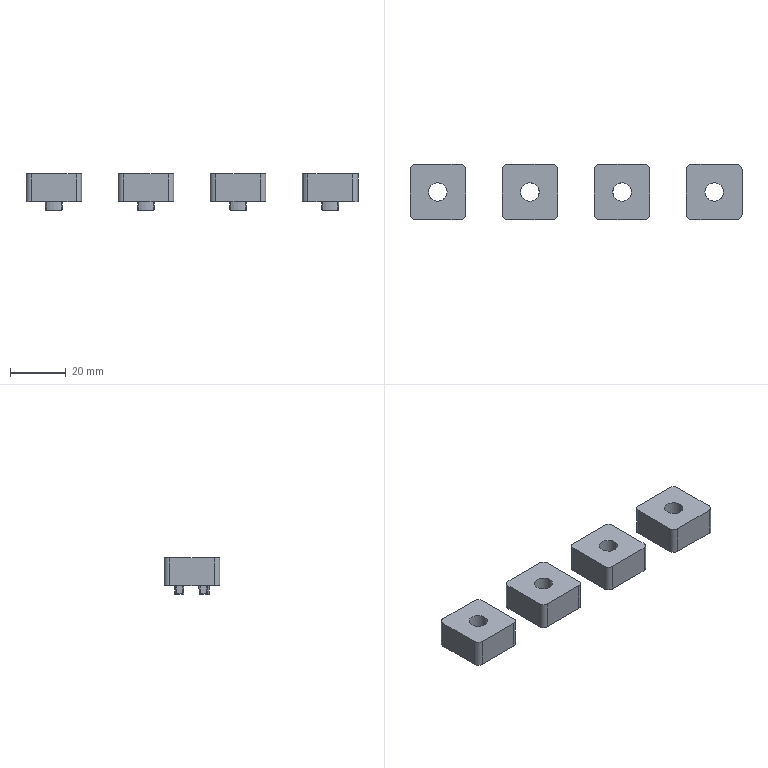NC program | NX | posted with a generic post | part box 118.91 x 19.91 x 13 mm
Whole program:
N10 G17 G21 G94 G90
(FLOOR_WALL_COPY , TOOL : D80)
N12 T19 M6
N14 G54
N16 G17 G0 G90 X-102.455 Y0. S6500 M3
N18 G43 Z30. H19
N20 Z9.
N22 G94 G1 Z6. F1500.
N24 X-99.455
N26 X99.455
N28 X102.455
N30 Z9.
N32 G0 Z30.
N34 X-102.455
N36 Z8.
N38 G1 Z5.
N40 X-99.455
N42 X99.455
N44 X102.455
N46 Z8.
N48 G0 Z30.
N50 X-102.455
N52 Z7.
N54 G1 Z4.
N56 X-99.455
N58 X99.455
N60 X102.455
N62 Z7.
N64 G0 Z30.
N66 X-102.455
N68 Z6.
N70 G1 Z3.
N72 X-99.455
N74 X99.455
N76 X102.455
N78 Z6.
N80 G0 Z30.
N82 X-102.455
N84 Z5.
N86 G1 Z2.
N88 X-99.455
N90 X99.455
N92 X102.455
N94 Z5.
N96 G0 Z30.
N98 X-102.455
N100 Z4.
N102 G1 Z1.
N104 X-99.455
N106 X99.455
N108 X102.455
N110 Z4.
N112 G0 Z30.
N114 X-102.455
N116 Z3.
N118 G1 Z0.
N120 X-99.455
N122 X99.455
N124 X102.455
N126 Z3.
N128 G0 Z30.
N130 M5
(PLANAR_MILL_COPY_COPY_COPY_COPY , TOOL : D6A45)
N132 T01 M6
N134 G54
N136 G17 G0 G90 X-60.855 Y-0.866 S9500 M3
N138 G43 Z30. H1
N140 Z0.5
N142 G94 G1 Z-1. F1250.
N144 G3 X-60.355 Y0. R1.
N146 G1 Y8.
N148 G2 X-57.5 Y10.855 R2.855
N150 G1 X-41.5
N152 G2 X-38.645 Y8. R2.855
N154 G1 Y-8.
N156 G2 X-41.5 Y-10.855 R2.855
N158 G1 X-57.5
N160 G2 X-60.355 Y-8. R2.855
N162 G1 Y0.
N164 G3 X-60.855 Y0.866 R1.
N166 G1 Z0.5
N168 G0 Z30.
N170 X-51.4
N172 Z0.5
N174 G1 Z-1.
N176 G3 X-51.9 Y0. R1.
N178 X-49.5 Y-2.4 R2.4
N180 X-51.9 Y0. R-2.4
N182 X-51.4 Y-0.866 R1.
N184 G1 Z0.5
N186 G0 Z30.
N188 X-17.366 Y11.355
N190 Z0.5
N192 G1 Z-1.
N194 G3 X-16.5 Y10.855 R1.
N196 G1 X-8.5
N198 G2 X-5.645 Y8. R2.855
N200 G1 Y-8.
N202 G2 X-8.5 Y-10.855 R2.855
N204 G1 X-24.5
N206 G2 X-27.355 Y-8. R2.855
N208 G1 Y8.
N210 G2 X-24.5 Y10.855 R2.855
N212 G1 X-16.5
N214 G3 X-15.634 Y11.355 R1.
N216 G1 Z0.5
N218 G0 Z30.
N220 Y1.9
N222 Z0.5
N224 G1 Z-1.
N226 G3 X-16.5 Y2.4 R1.
N228 X-18.9 Y0. R2.4
N230 X-16.5 Y2.4 R-2.4
N232 X-17.366 Y1.9 R1.
N234 G1 Z0.5
N236 G0 Z30.
N238 X17.366 Y-11.355
N240 Z0.5
N242 G1 Z-1.
N244 G3 X16.5 Y-10.855 R1.
N246 G1 X8.5
N248 G2 X5.645 Y-8. R2.855
N250 G1 Y8.
N252 G2 X8.5 Y10.855 R2.855
N254 G1 X24.5
N256 G2 X27.355 Y8. R2.855
N258 G1 Y-8.
N260 G2 X24.5 Y-10.855 R2.855
N262 G1 X16.5
N264 G3 X15.634 Y-11.355 R1.
N266 G1 Z0.5
N268 G0 Z30.
N270 Y-1.9
N272 Z0.5
N274 G1 Z-1.
N276 G3 X16.5 Y-2.4 R1.
N278 X18.9 Y0. R2.4
N280 X16.5 Y-2.4 R-2.4
N282 X17.366 Y-1.9 R1.
N284 G1 Z0.5
N286 G0 Z30.
N288 X50.366 Y-11.355
N290 Z0.5
N292 G1 Z-1.
N294 G3 X49.5 Y-10.855 R1.
N296 G1 X41.5
N298 G2 X38.645 Y-8. R2.855
N300 G1 Y8.
N302 G2 X41.5 Y10.855 R2.855
N304 G1 X57.5
N306 G2 X60.355 Y8. R2.855
N308 G1 Y-8.
N310 G2 X57.5 Y-10.855 R2.855
N312 G1 X49.5
N314 G3 X48.634 Y-11.355 R1.
N316 G1 Z0.5
N318 G0 Z30.
N320 Y-1.9
N322 Z0.5
N324 G1 Z-1.
N326 G3 X49.5 Y-2.4 R1.
N328 X51.9 Y0. R2.4
N330 X49.5 Y-2.4 R-2.4
N332 X50.366 Y-1.9 R1.
N334 G1 Z0.5
N336 G0 Z30.
N338 M5
N340 M2